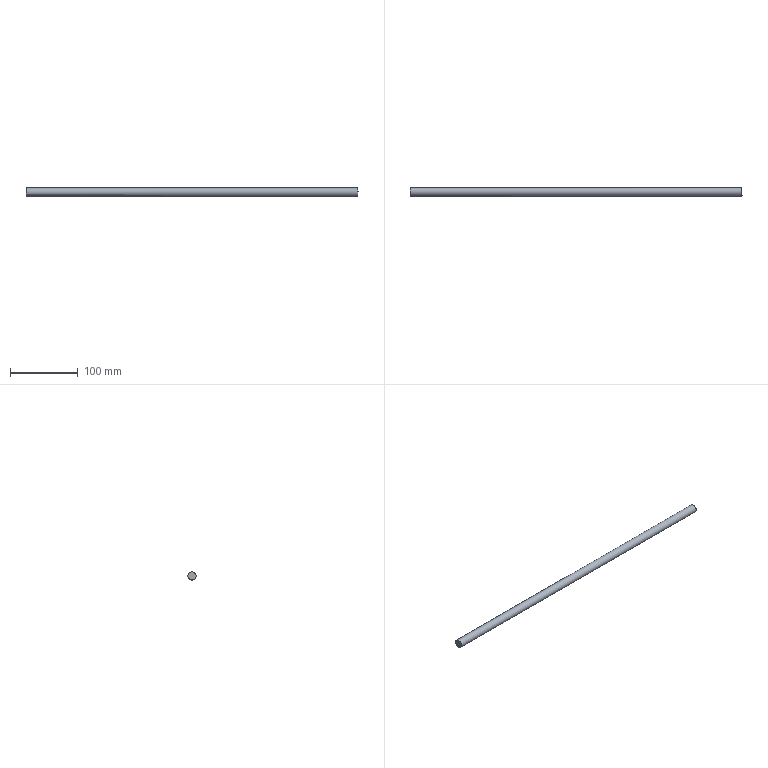Part | STEP file | solid 184 | 1 solid | 4 faces | box 489.684 x 12 x 12 mm | volume 55371 mm3 | plane 2 | cylinder 1 | torus 1 | commonest cylinder face diameters 12 x1